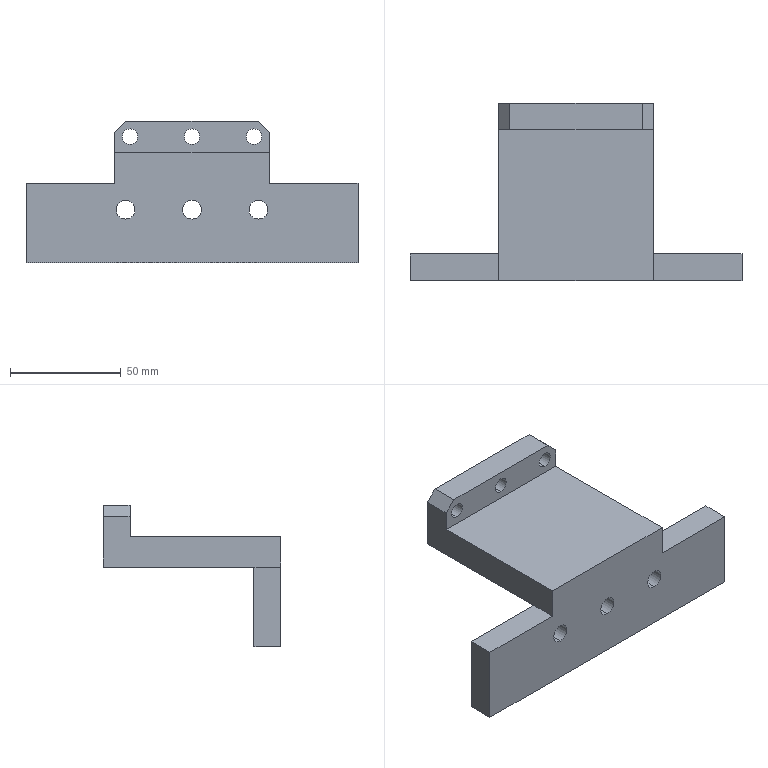NC program | NX | posted with a generic post | part box 150 x 80 x 64 mm
Whole program:
N10 G17 G21 G94 G90
(DRILLING , TOOL : D6A45)
N12 T07 M6
N14 G54
N16 G17 G0 G90 X28. Y25. B0. C0. S5000 M3
N18 G43 Z30. H7
N20 G94 G81 G98 Z-1. F250. R3.
N22 X0.
N24 X-28.
N26 X-30. Y-8. Z-69. R-65.
N28 X0.
N30 X30.
N32 G80
N34 G0 X30. Y-8. Z30.
N36 M5
N38 M2